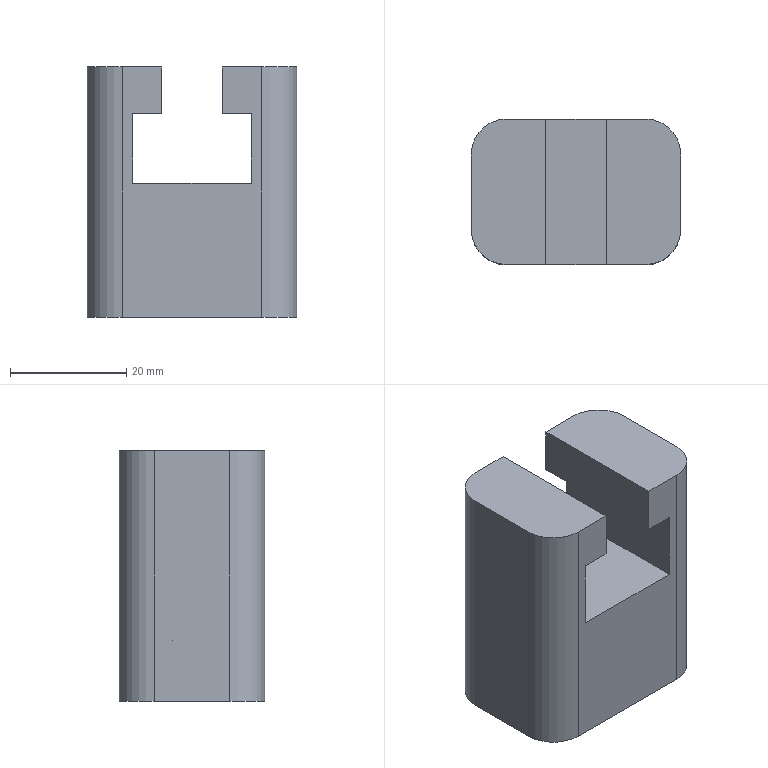Part | STEP file | solid 126 | 1 solid | 32 faces | box 36 x 25 x 43 mm | volume 28272 mm3 | plane 23 | cylinder 6 | other 2 | cone 1 | commonest cylinder face diameters 12 x4 6.7 x1 8 x1